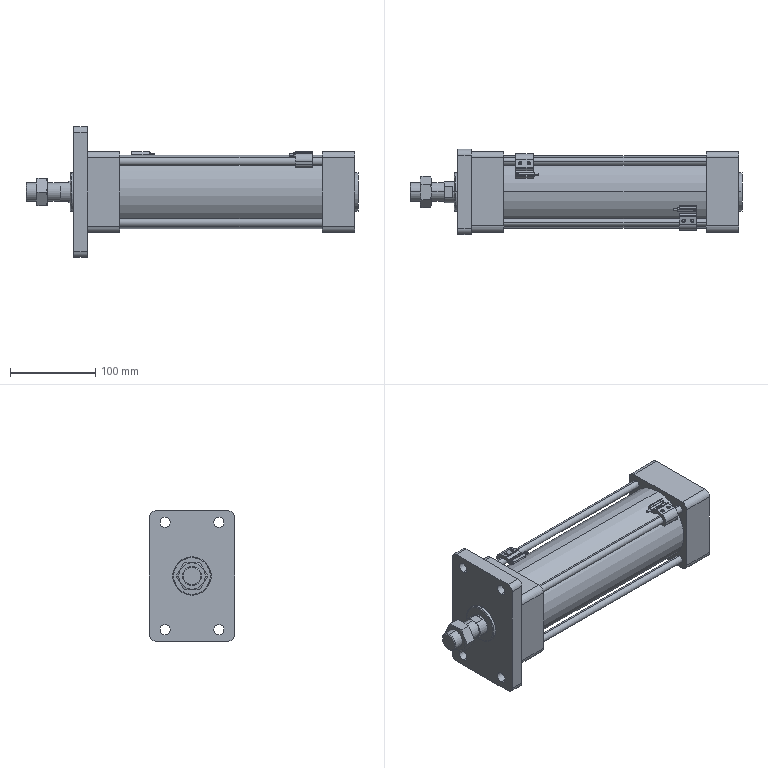Part | SolidWorks | features BaseBody 8 | 8 solids | 384 faces | box 390 x 100 x 153 mm | volume 1487562 mm3 | plane 193 | cylinder 155 | cone 34 | spline 2 | commonest cylinder face diameters 12 x27 4 x22 8.376 x16 11 x16 2 x9 9 x8